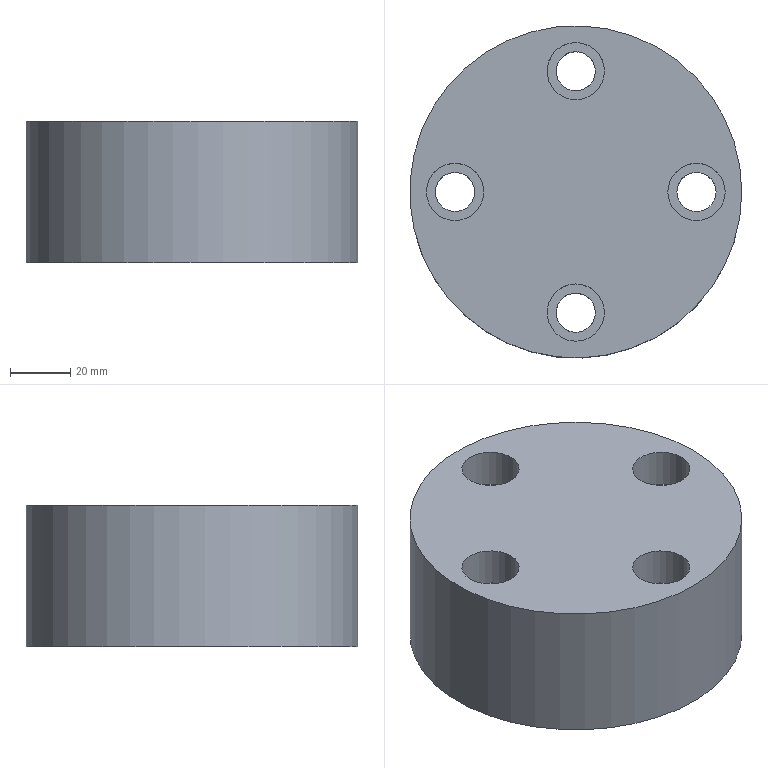Part | NX | 1 solid | 15 faces | box 110 x 110 x 47 mm | volume 413861 mm3 | cylinder 9 | plane 6 | commonest cylinder face diameters 13 x4 19 x4 110 x1
STEP:
#1=CARTESIAN_POINT('',(0.,-46.5,-47.));
#2=VERTEX_POINT('',#1);
#3=CARTESIAN_POINT('',(0.,-40.,-47.));
#4=DIRECTION('',(0.,0.,1.));
#5=DIRECTION('',(0.,-1.,0.));
#6=AXIS2_PLACEMENT_3D('',#3,#4,#5);
#7=CIRCLE('',#6,6.5);
#8=EDGE_CURVE('',#2,#2,#7,.T.);
#9=ORIENTED_EDGE('',*,*,#8,.F.);
#10=EDGE_LOOP('',(#9));
#11=FACE_BOUND('',#10,.T.);
#12=CARTESIAN_POINT('',(6.5,-40.,-13.));
#13=VERTEX_POINT('',#12);
#14=CARTESIAN_POINT('',(0.,-40.,-13.));
#15=DIRECTION('',(0.,0.,1.));
#16=DIRECTION('',(1.,0.,0.));
#17=AXIS2_PLACEMENT_3D('',#14,#15,#16);
#18=CIRCLE('',#17,6.5);
#19=EDGE_CURVE('',#13,#13,#18,.F.);
#20=ORIENTED_EDGE('',*,*,#19,.F.);
#21=EDGE_LOOP('',(#20));
#22=FACE_BOUND('',#21,.T.);
#23=CARTESIAN_POINT('',(0.,-40.,-47.));
#24=DIRECTION('',(0.,0.,1.));
#25=DIRECTION('',(1.,0.,0.));
#26=AXIS2_PLACEMENT_3D('',#23,#24,#25);
#27=CYLINDRICAL_SURFACE('',#26,6.5);
#28=ADVANCED_FACE('',(#11,#22),#27,.F.);
#29=CARTESIAN_POINT('',(0.,46.5,-47.));
#30=VERTEX_POINT('',#29);
#31=CARTESIAN_POINT('',(0.,40.,-47.));
#32=DIRECTION('',(0.,0.,1.));
#33=DIRECTION('',(0.,1.,0.));
#34=AXIS2_PLACEMENT_3D('',#31,#32,#33);
#35=CIRCLE('',#34,6.5);
#36=EDGE_CURVE('',#30,#30,#35,.T.);
#37=ORIENTED_EDGE('',*,*,#36,.F.);
#38=EDGE_LOOP('',(#37));
#39=FACE_BOUND('',#38,.T.);
#40=CARTESIAN_POINT('',(6.5,40.,-13.));
#41=VERTEX_POINT('',#40);
#42=CARTESIAN_POINT('',(0.,40.,-13.));
#43=DIRECTION('',(0.,0.,1.));
#44=DIRECTION('',(1.,0.,0.));
#45=AXIS2_PLACEMENT_3D('',#42,#43,#44);
#46=CIRCLE('',#45,6.5);
#47=EDGE_CURVE('',#41,#41,#46,.F.);
#48=ORIENTED_EDGE('',*,*,#47,.F.);
#49=EDGE_LOOP('',(#48));
#50=FACE_BOUND('',#49,.T.);
#51=CARTESIAN_POINT('',(0.,40.,-47.));
#52=DIRECTION('',(0.,0.,1.));
#53=DIRECTION('',(1.,0.,0.));
#54=AXIS2_PLACEMENT_3D('',#51,#52,#53);
#55=CYLINDRICAL_SURFACE('',#54,6.5);
#56=ADVANCED_FACE('',(#39,#50),#55,.F.);
#57=CARTESIAN_POINT('',(46.5,0.,-47.));
#58=VERTEX_POINT('',#57);
#59=CARTESIAN_POINT('',(40.,0.,-47.));
#60=DIRECTION('',(0.,0.,1.));
#61=DIRECTION('',(1.,0.,0.));
#62=AXIS2_PLACEMENT_3D('',#59,#60,#61);
#63=CIRCLE('',#62,6.5);
#64=EDGE_CURVE('',#58,#58,#63,.T.);
#65=ORIENTED_EDGE('',*,*,#64,.F.);
#66=EDGE_LOOP('',(#65));
#67=FACE_BOUND('',#66,.T.);
#68=CARTESIAN_POINT('',(46.5,0.,-13.));
#69=VERTEX_POINT('',#68);
#70=CARTESIAN_POINT('',(40.,0.,-13.));
#71=DIRECTION('',(0.,0.,1.));
#72=DIRECTION('',(1.,0.,0.));
#73=AXIS2_PLACEMENT_3D('',#70,#71,#72);
#74=CIRCLE('',#73,6.5);
#75=EDGE_CURVE('',#69,#69,#74,.F.);
#76=ORIENTED_EDGE('',*,*,#75,.F.);
#77=EDGE_LOOP('',(#76));
#78=FACE_BOUND('',#77,.T.);
#79=CARTESIAN_POINT('',(40.,0.,-47.));
#80=DIRECTION('',(0.,0.,1.));
#81=DIRECTION('',(1.,0.,0.));
#82=AXIS2_PLACEMENT_3D('',#79,#80,#81);
#83=CYLINDRICAL_SURFACE('',#82,6.5);
#84=ADVANCED_FACE('',(#67,#78),#83,.F.);
#85=CARTESIAN_POINT('',(0.,49.5,0.));
#86=VERTEX_POINT('',#85);
#87=CARTESIAN_POINT('',(0.,40.,0.));
#88=DIRECTION('',(0.,0.,1.));
#89=DIRECTION('',(0.,1.,0.));
#90=AXIS2_PLACEMENT_3D('',#87,#88,#89);
#91=CIRCLE('',#90,9.5);
#92=EDGE_CURVE('',#86,#86,#91,.T.);
#93=ORIENTED_EDGE('',*,*,#92,.F.);
#94=EDGE_LOOP('',(#93));
#95=FACE_BOUND('',#94,.T.);
#96=CARTESIAN_POINT('',(55.,0.,0.));
#97=VERTEX_POINT('',#96);
#98=CARTESIAN_POINT('',(0.,0.,0.));
#99=DIRECTION('',(0.,0.,1.));
#100=DIRECTION('',(1.,0.,0.));
#101=AXIS2_PLACEMENT_3D('',#98,#99,#100);
#102=CIRCLE('',#101,55.);
#103=EDGE_CURVE('',#97,#97,#102,.T.);
#104=ORIENTED_EDGE('',*,*,#103,.T.);
#105=EDGE_LOOP('',(#104));
#106=FACE_BOUND('',#105,.T.);
#107=CARTESIAN_POINT('',(-49.5,0.,0.));
#108=VERTEX_POINT('',#107);
#109=CARTESIAN_POINT('',(-40.,0.,0.));
#110=DIRECTION('',(0.,0.,-1.));
#111=DIRECTION('',(-1.,0.,0.));
#112=AXIS2_PLACEMENT_3D('',#109,#110,#111);
#113=CIRCLE('',#112,9.5);
#114=EDGE_CURVE('',#108,#108,#113,.T.);
#115=ORIENTED_EDGE('',*,*,#114,.T.);
#116=EDGE_LOOP('',(#115));
#117=FACE_BOUND('',#116,.T.);
#118=CARTESIAN_POINT('',(0.,-49.5,0.));
#119=VERTEX_POINT('',#118);
#120=CARTESIAN_POINT('',(0.,-40.,0.));
#121=DIRECTION('',(0.,0.,1.));
#122=DIRECTION('',(0.,-1.,0.));
#123=AXIS2_PLACEMENT_3D('',#120,#121,#122);
#124=CIRCLE('',#123,9.5);
#125=EDGE_CURVE('',#119,#119,#124,.T.);
#126=ORIENTED_EDGE('',*,*,#125,.F.);
#127=EDGE_LOOP('',(#126));
#128=FACE_BOUND('',#127,.T.);
#129=CARTESIAN_POINT('',(49.5,0.,0.));
#130=VERTEX_POINT('',#129);
#131=CARTESIAN_POINT('',(40.,0.,0.));
#132=DIRECTION('',(0.,0.,1.));
#133=DIRECTION('',(1.,0.,0.));
#134=AXIS2_PLACEMENT_3D('',#131,#132,#133);
#135=CIRCLE('',#134,9.5);
#136=EDGE_CURVE('',#130,#130,#135,.T.);
#137=ORIENTED_EDGE('',*,*,#136,.F.);
#138=EDGE_LOOP('',(#137));
#139=FACE_BOUND('',#138,.T.);
#140=CARTESIAN_POINT('',(20.,0.,0.));
#141=DIRECTION('',(0.,0.,1.));
#142=DIRECTION('',(1.,0.,0.));
#143=AXIS2_PLACEMENT_3D('',#140,#141,#142);
#144=PLANE('',#143);
#145=ADVANCED_FACE('',(#95,#106,#117,#128,#139),#144,.T.);
#146=CARTESIAN_POINT('',(55.,0.,-47.));
#147=VERTEX_POINT('',#146);
#148=CARTESIAN_POINT('',(0.,0.,-47.));
#149=DIRECTION('',(0.,0.,1.));
#150=DIRECTION('',(1.,0.,0.));
#151=AXIS2_PLACEMENT_3D('',#148,#149,#150);
#152=CIRCLE('',#151,55.);
#153=EDGE_CURVE('',#147,#147,#152,.T.);
#154=ORIENTED_EDGE('',*,*,#153,.T.);
#155=EDGE_LOOP('',(#154));
#156=FACE_BOUND('',#155,.T.);
#157=ORIENTED_EDGE('',*,*,#103,.F.);
#158=EDGE_LOOP('',(#157));
#159=FACE_BOUND('',#158,.T.);
#160=CARTESIAN_POINT('',(0.,0.,-47.));
#161=DIRECTION('',(0.,0.,1.));
#162=DIRECTION('',(1.,0.,0.));
#163=AXIS2_PLACEMENT_3D('',#160,#161,#162);
#164=CYLINDRICAL_SURFACE('',#163,55.);
#165=ADVANCED_FACE('',(#156,#159),#164,.T.);
#166=CARTESIAN_POINT('',(-46.5,0.,-13.));
#167=VERTEX_POINT('',#166);
#168=CARTESIAN_POINT('',(-40.,0.,-13.));
#169=DIRECTION('',(0.,0.,-1.));
#170=DIRECTION('',(-1.,0.,0.));
#171=AXIS2_PLACEMENT_3D('',#168,#169,#170);
#172=CIRCLE('',#171,6.5);
#173=EDGE_CURVE('',#167,#167,#172,.F.);
#174=ORIENTED_EDGE('',*,*,#173,.T.);
#175=EDGE_LOOP('',(#174));
#176=FACE_BOUND('',#175,.T.);
#177=CARTESIAN_POINT('',(-46.5,0.,-47.));
#178=VERTEX_POINT('',#177);
#179=CARTESIAN_POINT('',(-40.,0.,-47.));
#180=DIRECTION('',(0.,0.,1.));
#181=DIRECTION('',(-1.,0.,0.));
#182=AXIS2_PLACEMENT_3D('',#179,#180,#181);
#183=CIRCLE('',#182,6.5);
#184=EDGE_CURVE('',#178,#178,#183,.T.);
#185=ORIENTED_EDGE('',*,*,#184,.F.);
#186=EDGE_LOOP('',(#185));
#187=FACE_BOUND('',#186,.T.);
#188=CARTESIAN_POINT('',(-40.,0.,-47.));
#189=DIRECTION('',(0.,0.,1.));
#190=DIRECTION('',(1.,0.,0.));
#191=AXIS2_PLACEMENT_3D('',#188,#189,#190);
#192=CYLINDRICAL_SURFACE('',#191,6.5);
#193=ADVANCED_FACE('',(#176,#187),#192,.F.);
#194=ORIENTED_EDGE('',*,*,#153,.F.);
#195=EDGE_LOOP('',(#194));
#196=FACE_BOUND('',#195,.T.);
#197=ORIENTED_EDGE('',*,*,#64,.T.);
#198=EDGE_LOOP('',(#197));
#199=FACE_BOUND('',#198,.T.);
#200=ORIENTED_EDGE('',*,*,#36,.T.);
#201=EDGE_LOOP('',(#200));
#202=FACE_BOUND('',#201,.T.);
#203=ORIENTED_EDGE('',*,*,#8,.T.);
#204=EDGE_LOOP('',(#203));
#205=FACE_BOUND('',#204,.T.);
#206=ORIENTED_EDGE('',*,*,#184,.T.);
#207=EDGE_LOOP('',(#206));
#208=FACE_BOUND('',#207,.T.);
#209=CARTESIAN_POINT('',(20.,0.,-47.));
#210=DIRECTION('',(0.,0.,1.));
#211=DIRECTION('',(1.,0.,0.));
#212=AXIS2_PLACEMENT_3D('',#209,#210,#211);
#213=PLANE('',#212);
#214=ADVANCED_FACE('',(#196,#199,#202,#205,#208),#213,.F.);
#215=CARTESIAN_POINT('',(-49.5,0.,-13.));
#216=VERTEX_POINT('',#215);
#217=CARTESIAN_POINT('',(-40.,0.,-13.));
#218=DIRECTION('',(0.,0.,-1.));
#219=DIRECTION('',(-1.,0.,0.));
#220=AXIS2_PLACEMENT_3D('',#217,#218,#219);
#221=CIRCLE('',#220,9.5);
#222=EDGE_CURVE('',#216,#216,#221,.F.);
#223=ORIENTED_EDGE('',*,*,#222,.T.);
#224=EDGE_LOOP('',(#223));
#225=FACE_BOUND('',#224,.T.);
#226=ORIENTED_EDGE('',*,*,#173,.F.);
#227=EDGE_LOOP('',(#226));
#228=FACE_BOUND('',#227,.T.);
#229=CARTESIAN_POINT('',(-40.,0.,-13.));
#230=DIRECTION('',(0.,0.,-1.));
#231=DIRECTION('',(-1.,0.,0.));
#232=AXIS2_PLACEMENT_3D('',#229,#230,#231);
#233=PLANE('',#232);
#234=ADVANCED_FACE('',(#225,#228),#233,.F.);
#235=ORIENTED_EDGE('',*,*,#222,.F.);
#236=EDGE_LOOP('',(#235));
#237=FACE_BOUND('',#236,.T.);
#238=ORIENTED_EDGE('',*,*,#114,.F.);
#239=EDGE_LOOP('',(#238));
#240=FACE_BOUND('',#239,.T.);
#241=CARTESIAN_POINT('',(-40.,0.,-13.));
#242=DIRECTION('',(0.,0.,1.));
#243=DIRECTION('',(1.,0.,0.));
#244=AXIS2_PLACEMENT_3D('',#241,#242,#243);
#245=CYLINDRICAL_SURFACE('',#244,9.5);
#246=ADVANCED_FACE('',(#237,#240),#245,.F.);
#247=CARTESIAN_POINT('',(0.,-49.5,-13.));
#248=VERTEX_POINT('',#247);
#249=CARTESIAN_POINT('',(0.,-40.,-13.));
#250=DIRECTION('',(0.,0.,1.));
#251=DIRECTION('',(0.,-1.,0.));
#252=AXIS2_PLACEMENT_3D('',#249,#250,#251);
#253=CIRCLE('',#252,9.5);
#254=EDGE_CURVE('',#248,#248,#253,.F.);
#255=ORIENTED_EDGE('',*,*,#254,.F.);
#256=EDGE_LOOP('',(#255));
#257=FACE_BOUND('',#256,.T.);
#258=ORIENTED_EDGE('',*,*,#19,.T.);
#259=EDGE_LOOP('',(#258));
#260=FACE_BOUND('',#259,.T.);
#261=CARTESIAN_POINT('',(0.,-40.,-13.));
#262=DIRECTION('',(0.,0.,1.));
#263=DIRECTION('',(1.,0.,0.));
#264=AXIS2_PLACEMENT_3D('',#261,#262,#263);
#265=PLANE('',#264);
#266=ADVANCED_FACE('',(#257,#260),#265,.T.);
#267=ORIENTED_EDGE('',*,*,#254,.T.);
#268=EDGE_LOOP('',(#267));
#269=FACE_BOUND('',#268,.T.);
#270=ORIENTED_EDGE('',*,*,#125,.T.);
#271=EDGE_LOOP('',(#270));
#272=FACE_BOUND('',#271,.T.);
#273=CARTESIAN_POINT('',(0.,-40.,-13.));
#274=DIRECTION('',(0.,0.,1.));
#275=DIRECTION('',(1.,0.,0.));
#276=AXIS2_PLACEMENT_3D('',#273,#274,#275);
#277=CYLINDRICAL_SURFACE('',#276,9.5);
#278=ADVANCED_FACE('',(#269,#272),#277,.F.);
#279=CARTESIAN_POINT('',(0.,49.5,-13.));
#280=VERTEX_POINT('',#279);
#281=CARTESIAN_POINT('',(0.,40.,-13.));
#282=DIRECTION('',(0.,0.,1.));
#283=DIRECTION('',(0.,1.,0.));
#284=AXIS2_PLACEMENT_3D('',#281,#282,#283);
#285=CIRCLE('',#284,9.5);
#286=EDGE_CURVE('',#280,#280,#285,.F.);
#287=ORIENTED_EDGE('',*,*,#286,.F.);
#288=EDGE_LOOP('',(#287));
#289=FACE_BOUND('',#288,.T.);
#290=ORIENTED_EDGE('',*,*,#47,.T.);
#291=EDGE_LOOP('',(#290));
#292=FACE_BOUND('',#291,.T.);
#293=CARTESIAN_POINT('',(0.,40.,-13.));
#294=DIRECTION('',(0.,0.,1.));
#295=DIRECTION('',(1.,0.,0.));
#296=AXIS2_PLACEMENT_3D('',#293,#294,#295);
#297=PLANE('',#296);
#298=ADVANCED_FACE('',(#289,#292),#297,.T.);
#299=ORIENTED_EDGE('',*,*,#286,.T.);
#300=EDGE_LOOP('',(#299));
#301=FACE_BOUND('',#300,.T.);
#302=ORIENTED_EDGE('',*,*,#92,.T.);
#303=EDGE_LOOP('',(#302));
#304=FACE_BOUND('',#303,.T.);
#305=CARTESIAN_POINT('',(0.,40.,-13.));
#306=DIRECTION('',(0.,0.,1.));
#307=DIRECTION('',(1.,0.,0.));
#308=AXIS2_PLACEMENT_3D('',#305,#306,#307);
#309=CYLINDRICAL_SURFACE('',#308,9.5);
#310=ADVANCED_FACE('',(#301,#304),#309,.F.);
#311=CARTESIAN_POINT('',(49.5,0.,-13.));
#312=VERTEX_POINT('',#311);
#313=CARTESIAN_POINT('',(40.,0.,-13.));
#314=DIRECTION('',(0.,0.,1.));
#315=DIRECTION('',(1.,0.,0.));
#316=AXIS2_PLACEMENT_3D('',#313,#314,#315);
#317=CIRCLE('',#316,9.5);
#318=EDGE_CURVE('',#312,#312,#317,.F.);
#319=ORIENTED_EDGE('',*,*,#318,.F.);
#320=EDGE_LOOP('',(#319));
#321=FACE_BOUND('',#320,.T.);
#322=ORIENTED_EDGE('',*,*,#75,.T.);
#323=EDGE_LOOP('',(#322));
#324=FACE_BOUND('',#323,.T.);
#325=CARTESIAN_POINT('',(40.,0.,-13.));
#326=DIRECTION('',(0.,0.,1.));
#327=DIRECTION('',(1.,0.,0.));
#328=AXIS2_PLACEMENT_3D('',#325,#326,#327);
#329=PLANE('',#328);
#330=ADVANCED_FACE('',(#321,#324),#329,.T.);
#331=ORIENTED_EDGE('',*,*,#318,.T.);
#332=EDGE_LOOP('',(#331));
#333=FACE_BOUND('',#332,.T.);
#334=ORIENTED_EDGE('',*,*,#136,.T.);
#335=EDGE_LOOP('',(#334));
#336=FACE_BOUND('',#335,.T.);
#337=CARTESIAN_POINT('',(40.,0.,-13.));
#338=DIRECTION('',(0.,0.,1.));
#339=DIRECTION('',(1.,0.,0.));
#340=AXIS2_PLACEMENT_3D('',#337,#338,#339);
#341=CYLINDRICAL_SURFACE('',#340,9.5);
#342=ADVANCED_FACE('',(#333,#336),#341,.F.);
#343=CLOSED_SHELL('',(#28,#56,#84,#145,#165,#193,#214,#234,#246,#266,#278,#298,#310,#330,#342));
#344=MANIFOLD_SOLID_BREP('',#343);
#345=(LENGTH_UNIT()NAMED_UNIT(*)SI_UNIT(.MILLI.,.METRE.));
#346=UNCERTAINTY_MEASURE_WITH_UNIT(LENGTH_MEASURE(0.00001),#345,'','');
#347=(NAMED_UNIT(*)PLANE_ANGLE_UNIT()SI_UNIT($,.RADIAN.));
#348=(NAMED_UNIT(*)SI_UNIT($,.STERADIAN.)SOLID_ANGLE_UNIT());
#349=(GEOMETRIC_REPRESENTATION_CONTEXT(3)GLOBAL_UNCERTAINTY_ASSIGNED_CONTEXT((#346))GLOBAL_UNIT_ASSIGNED_CONTEXT((#345,#347,#348))REPRESENTATION_CONTEXT('',''));
#350=ADVANCED_BREP_SHAPE_REPRESENTATION('',(#344),#349);